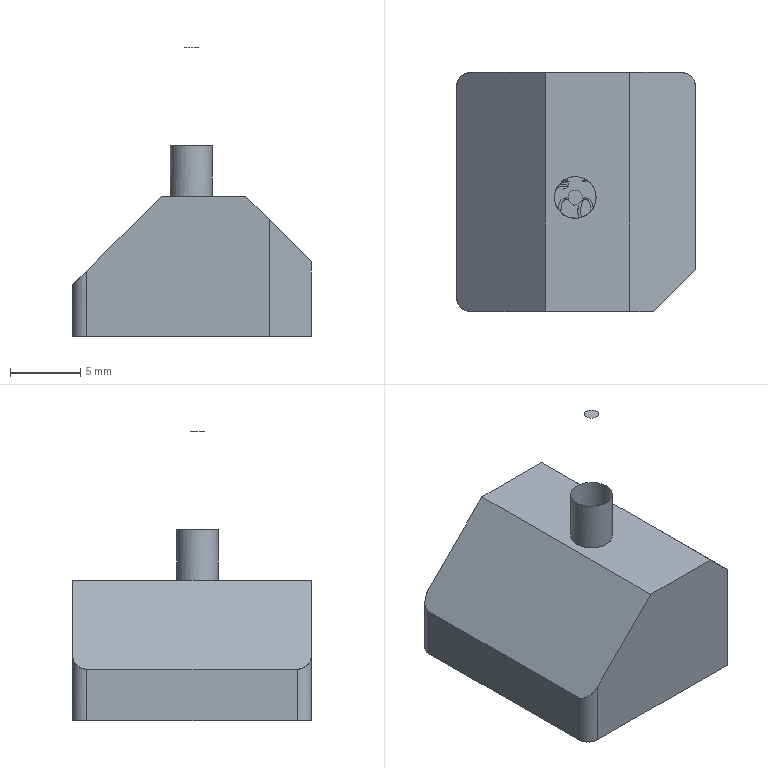NC program | PowerMill | posted with a generic post | part box 17 x 17 x 20.603 mm
Lines 3962 to 5007 of 42778:
N4059 M6
N4060 S18000 M03
N4061 G00 G90 X0.002 Y0.0
N4062 G43 Z10.803 H14
N4063
N4064 G05 P10000 R8
N4065 X1.2168 Y-3.1988
N4066 Z0.8074
N4067 G01 Z-0.3926 F1200.0
N4068 X1.1992 Y-3.1296 F2000.0
N4069 X1.174 Y-3.0627
N4070 X1.1415 Y-2.9991
N4071 X1.102 Y-2.9395
N4072 X1.0562 Y-2.8847
N4073 X1.0046 Y-2.8353
N4074 X0.9478 Y-2.792
N4075 X0.8865 Y-2.7553
N4076 X0.8215 Y-2.7256
N4077 X0.7536 Y-2.7034
N4078 X0.6836 Y-2.6889
N4079 X0.6124 Y-2.6823
N4080 X0.541 Y-2.6836
N4081 X0.4702 Y-2.6929
N4082 X0.4657 Y-2.6938
N4083 X0.3401 Y-2.7184
N4084 X0.2083 Y-2.7366
N4085 X0.0731 Y-2.7478
N4086 X-0.0548 Y-2.7513
N4087 X-0.1828 Y-2.7476
N4088 X-0.3196 Y-2.7359
N4089 X-0.4555 Y-2.7162
N4090 X-0.5901 Y-2.6887
N4091 X-0.7228 Y-2.6534
N4092 X-0.8532 Y-2.6105
N4093 X-0.9809 Y-2.56
N4094 X-1.1048 Y-2.5025
N4095 X-1.2252 Y-2.4378
N4096 X-1.3415 Y-2.3664
N4097 X-1.4534 Y-2.2882
N4098 X-1.5606 Y-2.2037
N4099 X-1.6629 Y-2.113
N4100 X-1.7598 Y-2.0163
N4101 X-1.8511 Y-1.914
N4102 X-1.9364 Y-1.8064
N4103 X-2.0154 Y-1.694
N4104 X-2.0876 Y-1.5772
N4105 X-2.1529 Y-1.4566
N4106 X-2.211 Y-1.3325
N4107 X-2.2616 Y-1.2056
N4108 X-2.3048 Y-1.0759
N4109 X-2.3403 Y-0.944
N4110 X-2.3672 Y-0.8149
N4111 X-2.3868 Y-0.6833
N4112 X-2.3991 Y-0.5473
N4113 X-2.4036 Y-0.4091
N4114 X-2.4002 Y-0.2725
N4115 X-2.3892 Y-0.1398
N4116 X-2.371 Y-0.0105
N4117 X-2.3454 Y0.1205
N4118 X-2.3121 Y0.2505
N4119 X-2.2717 Y0.3769
N4120 X-2.2247 Y0.4992
N4121 X-2.171 Y0.6193
N4122 X-2.1083 Y0.7407
N4123 X-2.0386 Y0.8582
N4124 X-1.9622 Y0.9715
N4125 X-1.8793 Y1.0801
N4126 X-1.7902 Y1.1838
N4127 X-1.6951 Y1.2823
N4128 X-1.5943 Y1.3751
N4129 X-1.4883 Y1.4619
N4130 X-1.3773 Y1.5424
N4131 X-1.262 Y1.6162
N4132 X-1.1426 Y1.6832
N4133 X-1.0197 Y1.743
N4134 X-0.8935 Y1.7956
N4135 X-0.7645 Y1.8407
N4136 X-0.6331 Y1.8783
N4137 X-0.4997 Y1.9082
N4138 X-0.3645 Y1.9303
N4139 X-0.2281 Y1.9446
N4140 X-0.0912 Y1.9509
N4141 X0.0459 Y1.9492
N4142 X0.1824 Y1.9395
N4143 X0.3181 Y1.9219
N4144 X0.4525 Y1.8964
N4145 X0.585 Y1.8632
N4146 X0.7152 Y1.8224
N4147 X0.8428 Y1.7741
N4148 X0.9676 Y1.7184
N4149 X1.089 Y1.6556
N4150 X1.2066 Y1.5857
N4151 X1.3201 Y1.509
N4152 X1.429 Y1.4258
N4153 X1.5329 Y1.3364
N4154 X1.6315 Y1.241
N4155 X1.7242 Y1.1402
N4156 X1.8108 Y1.0342
N4157 X1.891 Y0.9235
N4158 X1.9646 Y0.8085
N4159 X2.0312 Y0.6894
N4160 X2.0909 Y0.5668
N4161 X2.1433 Y0.441
N4162 X2.1883 Y0.3124
N4163 X2.2259 Y0.1811
N4164 X2.2559 Y0.0475
N4165 X2.2781 Y-0.0877
N4166 X2.2924 Y-0.2239
N4167 X2.2987 Y-0.3607
N4168 X2.297 Y-0.4977
N4169 X2.2873 Y-0.6344
N4170 X2.2697 Y-0.7703
N4171 X2.2442 Y-0.9049
N4172 X2.2109 Y-1.0377
N4173 X2.1699 Y-1.1684
N4174 X2.1213 Y-1.2965
N4175 X2.0654 Y-1.4214
N4176 X2.0024 Y-1.5429
N4177 X1.9324 Y-1.6605
N4178 X1.8557 Y-1.7738
N4179 X1.7725 Y-1.8824
N4180 X1.6832 Y-1.9861
N4181 X1.5878 Y-2.0845
N4182 X1.4868 Y-2.1772
N4183 X1.3805 Y-2.264
N4184 X1.2693 Y-2.3444
N4185 X1.1538 Y-2.4182
N4186 X1.0342 Y-2.485
N4187 X0.9111 Y-2.5448
N4188 X0.7847 Y-2.5972
N4189 X0.6555 Y-2.6423
N4190 X0.5239 Y-2.6798
N4191 X0.4657 Y-2.6938
N4192 X0.3973 Y-2.7143
N4193 X0.3316 Y-2.7423
N4194 X0.2694 Y-2.7775
N4195 X0.2115 Y-2.8194
N4196 X0.1587 Y-2.8675
N4197 X0.1115 Y-2.9212
N4198 X0.0707 Y-2.9798
N4199 X0.0366 Y-3.0426
N4200 X0.0097 Y-3.1088
N4201 X-0.0096 Y-3.1775
N4202 X-0.0212 Y-3.2481
N4203 X-0.0248 Y-3.3195
N4204 X-0.0204 Y-3.3907
N4205 X-0.0081 Y-3.4611
N4206 X-0.0071 Y-3.4656
N4207 X1.2241 Y-3.1952 Z-0.4404
N4208 X1.2056 Y-3.1262
N4209 X1.1796 Y-3.0597
N4210 X1.1463 Y-2.9965
N4211 X1.1061 Y-2.9373
N4212 X1.0597 Y-2.8831
N4213 X1.0074 Y-2.8343
N4214 X0.9501 Y-2.7917
N4215 X0.8884 Y-2.7558
N4216 X0.823 Y-2.7269
N4217 X0.7549 Y-2.7055
N4218 X0.6847 Y-2.6919
N4219 X0.6135 Y-2.6861
N4220 X0.5421 Y-2.6883
N4221 X0.4714 Y-2.6985
N4222 X0.4669 Y-2.6994
N4223 X0.3618 Y-2.7213
N4224 X0.226 Y-2.7415
N4225 X0.0894 Y-2.7537
N4226 X-0.0478 Y-2.7579
N4227 X-0.185 Y-2.7542
N4228 X-0.3217 Y-2.7424
N4229 X-0.4575 Y-2.7227
N4230 X-0.5916 Y-2.6953
N4231 X-0.7235 Y-2.6602
N4232 X-0.8531 Y-2.6177
N4233 X-0.98 Y-2.5677
N4234 X-1.1039 Y-2.5104
N4235 X-1.2244 Y-2.446
N4236 X-1.341 Y-2.3746
N4237 X-1.4535 Y-2.2965
N4238 X-1.5614 Y-2.2118
N4239 X-1.6642 Y-2.121
N4240 X-1.7617 Y-2.0242
N4241 X-1.8534 Y-1.9219
N4242 X-1.939 Y-1.8145
N4243 X-2.018 Y-1.7025
N4244 X-2.0904 Y-1.5862
N4245 X-2.1557 Y-1.466
N4246 X-2.214 Y-1.3424
N4247 X-2.2649 Y-1.2158
N4248 X-2.3083 Y-1.0865
N4249 X-2.3442 Y-0.9549
N4250 X-2.3725 Y-0.8213
N4251 X-2.3931 Y-0.6857
N4252 X-2.4058 Y-0.5492
N4253 X-2.4105 Y-0.412
N4254 X-2.4072 Y-0.2748
N4255 X-2.3959 Y-0.1382
N4256 X-2.3767 Y-0.0025
N4257 X-2.3497 Y0.1316
N4258 X-2.315 Y0.2638
N4259 X-2.2727 Y0.3938
N4260 X-2.223 Y0.5212
N4261 X-2.1658 Y0.6457
N4262 X-2.1015 Y0.7667
N4263 X-2.0302 Y0.8838
N4264 X-1.9522 Y0.9967
N4265 X-1.8677 Y1.105
N4266 X-1.777 Y1.2081
N4267 X-1.6807 Y1.3056
N4268 X-1.5789 Y1.3973
N4269 X-1.472 Y1.4828
N4270 X-1.3606 Y1.5618
N4271 X-1.2448 Y1.6342
N4272 X-1.1251 Y1.6997
N4273 X-1.0019 Y1.7581
N4274 X-0.8755 Y1.8093
N4275 X-0.7463 Y1.8532
N4276 X-0.6144 Y1.8897
N4277 X-0.4804 Y1.9187
N4278 X-0.3453 Y1.9397
N4279 X-0.2094 Y1.9529
N4280 X-0.0731 Y1.958
N4281 X0.0635 Y1.9552
N4282 X0.2001 Y1.9444
N4283 X0.3363 Y1.9256
N4284 X0.4719 Y1.8988
N4285 X0.6034 Y1.865
N4286 X0.7329 Y1.8235
N4287 X0.8602 Y1.7744
N4288 X0.9847 Y1.7178
N4289 X1.106 Y1.6538
N4290 X1.2238 Y1.5827
N4291 X1.3375 Y1.5048
N4292 X1.4453 Y1.4212
N4293 X1.5484 Y1.3313
N4294 X1.6461 Y1.2356
N4295 X1.7381 Y1.1342
N4296 X1.8243 Y1.0275
N4297 X1.9042 Y0.9158
N4298 X1.9776 Y0.7995
N4299 X2.044 Y0.6792
N4300 X2.1033 Y0.5553
N4301 X2.1553 Y0.4284
N4302 X2.1997 Y0.2989
N4303 X2.2364 Y0.1672
N4304 X2.2655 Y0.0335
N4305 X2.2868 Y-0.1019
N4306 X2.3001 Y-0.2384
N4307 X2.3056 Y-0.3755
N4308 X2.303 Y-0.5128
N4309 X2.2925 Y-0.6495
N4310 X2.274 Y-0.7854
N4311 X2.2476 Y-0.9199
N4312 X2.2135 Y-1.0527
N4313 X2.1718 Y-1.1829
N4314 X2.1226 Y-1.3107
N4315 X2.0661 Y-1.4354
N4316 X2.0024 Y-1.5566
N4317 X1.9318 Y-1.674
N4318 X1.8544 Y-1.7872
N4319 X1.7705 Y-1.8957
N4320 X1.6804 Y-1.9991
N4321 X1.5845 Y-2.0972
N4322 X1.4831 Y-2.1894
N4323 X1.3765 Y-2.2756
N4324 X1.2651 Y-2.3554
N4325 X1.1492 Y-2.4286
N4326 X1.0293 Y-2.4951
N4327 X0.9058 Y-2.5545
N4328 X0.7801 Y-2.6062
N4329 X0.6511 Y-2.6506
N4330 X0.5189 Y-2.6877
N4331 X0.4961 Y-2.6933
N4332 X0.4669 Y-2.6994
N4333 X0.3979 Y-2.7179
N4334 X0.3314 Y-2.7439
N4335 X0.2682 Y-2.7772
N4336 X0.209 Y-2.8174
N4337 X0.1548 Y-2.8638
N4338 X0.106 Y-2.9161
N4339 X0.0634 Y-2.9734
N4340 X0.0275 Y-3.0351
N4341 X-0.0014 Y-3.1005
N4342 X-0.0228 Y-3.1686
N4343 X-0.0365 Y-3.2388
N4344 X-0.0422 Y-3.31
N4345 X-0.04 Y-3.3814
N4346 X-0.0298 Y-3.4521
N4347 X-0.0289 Y-3.4566
N4348 X1.2313 Y-3.1926 Z-0.4882
N4349 X1.212 Y-3.1238
N4350 X1.1852 Y-3.0576
N4351 X1.1511 Y-2.9948
N4352 X1.1103 Y-2.9361
N4353 X1.0632 Y-2.8824
N4354 X1.0104 Y-2.8343
N4355 X0.9525 Y-2.7924
N4356 X0.8904 Y-2.7571
N4357 X0.8247 Y-2.7291
N4358 X0.7563 Y-2.7085
N4359 X0.686 Y-2.6956
N4360 X0.6147 Y-2.6907
N4361 X0.5433 Y-2.6938
N4362 X0.4728 Y-2.7047
N4363 X0.4683 Y-2.7057
N4364 X0.3906 Y-2.7229
N4365 X0.255 Y-2.7447
N4366 X0.1183 Y-2.7585
N4367 X-0.019 Y-2.7644
N4368 X-0.1565 Y-2.7623
N4369 X-0.2936 Y-2.7522
N4370 X-0.4299 Y-2.7342
N4371 X-0.5648 Y-2.7084
N4372 X-0.698 Y-2.6747
N4373 X-0.829 Y-2.6334
N4374 X-0.9574 Y-2.5845
N4375 X-1.0827 Y-2.5283
N4376 X-1.2046 Y-2.4648
N4377 X-1.3227 Y-2.3944
N4378 X-1.4365 Y-2.3172
N4379 X-1.5456 Y-2.2335
N4380 X-1.6496 Y-2.1437
N4381 X-1.7481 Y-2.048
N4382 X-1.841 Y-1.9468
N4383 X-1.9278 Y-1.8403
N4384 X-2.0083 Y-1.729
N4385 X-2.0822 Y-1.6132
N4386 X-2.1492 Y-1.4934
N4387 X-2.2092 Y-1.3698
N4388 X-2.2618 Y-1.243
N4389 X-2.3071 Y-1.1133
N4390 X-2.3447 Y-0.9812
N4391 X-2.3746 Y-0.847
N4392 X-2.3966 Y-0.7113
N4393 X-2.4108 Y-0.5747
N4394 X-2.4169 Y-0.4375
N4395 X-2.4151 Y-0.3001
N4396 X-2.4053 Y-0.1632
N4397 X-2.3876 Y-0.027
N4398 X-2.362 Y0.1076
N4399 X-2.3288 Y0.2404
N4400 X-2.2879 Y0.371
N4401 X-2.2396 Y0.499
N4402 X-2.184 Y0.624
N4403 X-2.1211 Y0.7457
N4404 X-2.0512 Y0.8637
N4405 X-1.9745 Y0.9775
N4406 X-1.8912 Y1.0868
N4407 X-1.8016 Y1.1912
N4408 X-1.7061 Y1.2902
N4409 X-1.6051 Y1.3835
N4410 X-1.499 Y1.4706
N4411 X-1.3881 Y1.5513
N4412 X-1.2729 Y1.6254
N4413 X-1.1537 Y1.6926
N4414 X-1.0308 Y1.7527
N4415 X-0.9046 Y1.8056
N4416 X-0.7755 Y1.8512
N4417 X-0.6442 Y1.8892
N4418 X-0.5097 Y1.9198
N4419 X-0.3741 Y1.9426
N4420 X-0.2376 Y1.9574
N4421 X-0.1006 Y1.9643
N4422 X0.0364 Y1.9631
N4423 X0.1731 Y1.954
N4424 X0.3092 Y1.9369
N4425 X0.4441 Y1.9119
N4426 X0.577 Y1.8794
N4427 X0.7078 Y1.8391
N4428 X0.8361 Y1.7914
N4429 X0.9614 Y1.7363
N4430 X1.0834 Y1.6741
N4431 X1.2016 Y1.6048
N4432 X1.3158 Y1.5286
N4433 X1.4255 Y1.4459
N4434 X1.5303 Y1.3569
N4435 X1.6298 Y1.2619
N4436 X1.7235 Y1.1613
N4437 X1.8112 Y1.0556
N4438 X1.8925 Y0.945
N4439 X1.9672 Y0.83
N4440 X2.035 Y0.7111
N4441 X2.0958 Y0.5885
N4442 X2.1493 Y0.4626
N4443 X2.1956 Y0.3338
N4444 X2.2343 Y0.2024
N4445 X2.2654 Y0.0688
N4446 X2.2887 Y-0.0664
N4447 X2.3041 Y-0.2027
N4448 X2.3116 Y-0.3396
N4449 X2.3111 Y-0.477
N4450 X2.3026 Y-0.6142
N4451 X2.2862 Y-0.7508
N4452 X2.2618 Y-0.8862
N4453 X2.2297 Y-1.0199
N4454 X2.1899 Y-1.1512
N4455 X2.1426 Y-1.28
N4456 X2.0878 Y-1.4059
N4457 X2.0259 Y-1.5283
N4458 X1.9568 Y-1.6471
N4459 X1.8809 Y-1.7617
N4460 X1.7985 Y-1.8717
N4461 X1.7098 Y-1.9767
N4462 X1.6152 Y-2.0765
N4463 X1.5148 Y-2.1706
N4464 X1.4092 Y-2.2587
N4465 X1.2987 Y-2.3405
N4466 X1.1837 Y-2.4157
N4467 X1.0645 Y-2.4842
N4468 X0.9416 Y-2.5456
N4469 X0.8159 Y-2.5996
N4470 X0.6871 Y-2.6462
N4471 X0.5555 Y-2.6853
N4472 X0.5248 Y-2.6932
N4473 X0.4683 Y-2.7057
N4474 X0.3995 Y-2.725
N4475 X0.3333 Y-2.7518
N4476 X0.2705 Y-2.7859
N4477 X0.2118 Y-2.8267
N4478 X0.1581 Y-2.8738
N4479 X0.11 Y-2.9266
N4480 X0.0681 Y-2.9845
N4481 X0.0328 Y-3.0466
N4482 X0.0048 Y-3.1123
N4483 X-0.0158 Y-3.1807
N4484 X-0.0287 Y-3.251
N4485 X-0.0336 Y-3.3223
N4486 X-0.0305 Y-3.3937
N4487 X-0.0195 Y-3.4642
N4488 X-0.0186 Y-3.4687
N4489 X1.2384 Y-3.1902 Z-0.536
N4490 X1.2183 Y-3.1217
N4491 X1.1907 Y-3.0558
N4492 X1.156 Y-2.9934
N4493 X1.1144 Y-2.9352
N4494 X1.0667 Y-2.882
N4495 X1.0134 Y-2.8345
N4496 X0.955 Y-2.7933
N4497 X0.8925 Y-2.7587
N4498 X0.8265 Y-2.7314
N4499 X0.7578 Y-2.7116
N4500 X0.6874 Y-2.6996
N4501 X0.616 Y-2.6955
N4502 X0.5447 Y-2.6994
N4503 X0.4743 Y-2.7112
N4504 X0.4698 Y-2.7122
N4505 X0.4181 Y-2.7243
N4506 X0.2828 Y-2.7476
N4507 X0.1464 Y-2.7631
N4508 X0.0091 Y-2.7706
N4509 X-0.1286 Y-2.7701
N4510 X-0.2662 Y-2.7617
N4511 X-0.403 Y-2.7452
N4512 X-0.5387 Y-2.7209
N4513 X-0.6715 Y-2.6891
N4514 X-0.8025 Y-2.6495
N4515 X-0.9315 Y-2.6023
N4516 X-1.0579 Y-2.5474
N4517 X-1.1811 Y-2.4852
N4518 X-1.3007 Y-2.4159
N4519 X-1.4159 Y-2.3399
N4520 X-1.5264 Y-2.2575
N4521 X-1.6317 Y-2.1691
N4522 X-1.7314 Y-2.075
N4523 X-1.8251 Y-1.9756
N4524 X-1.9127 Y-1.8711
N4525 X-1.9944 Y-1.7614
N4526 X-2.0699 Y-1.6464
N4527 X-2.1389 Y-1.5269
N4528 X-2.2011 Y-1.4033
N4529 X-2.2559 Y-1.2765
N4530 X-2.3031 Y-1.1472
N4531 X-2.3426 Y-1.016
N4532 X-2.3742 Y-0.8833
N4533 X-2.3983 Y-0.7477
N4534 X-2.4145 Y-0.6109
N4535 X-2.4228 Y-0.4735
N4536 X-2.423 Y-0.3357
N4537 X-2.4153 Y-0.1983
N4538 X-2.3996 Y-0.0614
N4539 X-2.376 Y0.0742
N4540 X-2.3447 Y0.2078
N4541 X-2.3057 Y0.3393
N4542 X-2.2593 Y0.4682
N4543 X-2.2054 Y0.5943
N4544 X-2.1443 Y0.7171
N4545 X-2.0762 Y0.8362
N4546 X-2.0011 Y0.9514
N4547 X-1.9194 Y1.0621
N4548 X-1.8314 Y1.168
N4549 X-1.7373 Y1.2687
N4550 X-1.6376 Y1.3636
N4551 X-1.5327 Y1.4526
N4552 X-1.4229 Y1.5352
N4553 X-1.3087 Y1.6113
N4554 X-1.1903 Y1.6805
N4555 X-1.0682 Y1.7427
N4556 X-0.9427 Y1.7978
N4557 X-0.8141 Y1.8455
N4558 X-0.6829 Y1.8858
N4559 X-0.5493 Y1.9185
N4560 X-0.4139 Y1.9435
N4561 X-0.2773 Y1.9606
N4562 X-0.1398 Y1.9697
N4563 X-0.0022 Y1.9708
N4564 X0.1352 Y1.964
N4565 X0.2718 Y1.9492
N4566 X0.4074 Y1.9265
N4567 X0.5414 Y1.8959
N4568 X0.6734 Y1.8576
N4569 X0.8031 Y1.8118
N4570 X0.9299 Y1.7584
N4571 X1.0533 Y1.6978
N4572 X1.1731 Y1.6302
N4573 X1.2888 Y1.5556
N4574 X1.4001 Y1.4745
N4575 X1.5065 Y1.387
N4576 X1.6075 Y1.2935
N4577 X1.7029 Y1.1944
N4578 X1.7925 Y1.09
N4579 X1.8757 Y0.9805
N4580 X1.9525 Y0.8664
N4581 X2.0226 Y0.748
N4582 X2.0857 Y0.6258
N4583 X2.1416 Y0.5001
N4584 X2.19 Y0.3714
N4585 X2.231 Y0.2402
N4586 X2.2643 Y0.1067
N4587 X2.2898 Y-0.0285
N4588 X2.3074 Y-0.165
N4589 X2.317 Y-0.3024
N4590 X2.3187 Y-0.44
N4591 X2.3124 Y-0.5774
N4592 X2.2982 Y-0.7142
N4593 X2.276 Y-0.8499
N4594 X2.246 Y-0.9841
N4595 X2.2083 Y-1.1164
N4596 X2.1629 Y-1.2462
N4597 X2.1101 Y-1.3733
N4598 X2.05 Y-1.497
N4599 X1.9829 Y-1.6171
N4600 X1.9088 Y-1.7331
N4601 X1.8282 Y-1.8446
N4602 X1.7411 Y-1.9513
N4603 X1.6481 Y-2.0527
N4604 X1.5494 Y-2.1485
N4605 X1.4453 Y-2.2385
N4606 X1.3361 Y-2.3222
N4607 X1.2226 Y-2.3993
N4608 X1.1042 Y-2.4702
N4609 X0.9828 Y-2.5336
N4610 X0.8581 Y-2.5898
N4611 X0.7302 Y-2.6386
N4612 X0.599 Y-2.6802
N4613 X0.5518 Y-2.6931
N4614 X0.4698 Y-2.7122
N4615 X0.4013 Y-2.7323
N4616 X0.3354 Y-2.7599
N4617 X0.273 Y-2.7947
N4618 X0.2148 Y-2.8362
N4619 X0.1616 Y-2.8839
N4620 X0.1141 Y-2.9373
N4621 X0.0729 Y-2.9956
N4622 X0.0383 Y-3.0582
N4623 X0.011 Y-3.1242
N4624 X-0.0088 Y-3.1928
N4625 X-0.0208 Y-3.2633
N4626 X-0.0249 Y-3.3346
N4627 X-0.021 Y-3.4059
N4628 X-0.0092 Y-3.4764
N4629 X-0.0082 Y-3.4808
N4630 X1.2448 Y-3.1895 Z-0.5838
N4631 X1.224 Y-3.1211
N4632 X1.1958 Y-3.0555
N4633 X1.1604 Y-2.9934
N4634 X1.1183 Y-2.9356
N4635 X1.07 Y-2.883
N4636 X1.0162 Y-2.836
N4637 X0.9575 Y-2.7953
N4638 X0.8946 Y-2.7614
N4639 X0.8283 Y-2.7348
N4640 X0.7595 Y-2.7156
N4641 X0.6889 Y-2.7043
N4642 X0.6175 Y-2.7009
N4643 X0.5463 Y-2.7055
N4644 X0.4759 Y-2.718
N4645 X0.4715 Y-2.7191
N4646 X0.4435 Y-2.7259
N4647 X0.308 Y-2.7507
N4648 X0.1712 Y-2.7676
N4649 X0.0336 Y-2.7765
N4650 X-0.1043 Y-2.7775
N4651 X-0.242 Y-2.7705
N4652 X-0.379 Y-2.7555
N4653 X-0.5149 Y-2.7326
N4654 X-0.6492 Y-2.7019
N4655 X-0.7815 Y-2.6635
N4656 X-0.9113 Y-2.6175
N4657 X-1.0382 Y-2.5641
N4658 X-1.1618 Y-2.5034
N4659 X-1.2818 Y-2.4356
N4660 X-1.3977 Y-2.3609
N4661 X-1.5091 Y-2.2797
N4662 X-1.6156 Y-2.1921
N4663 X-1.7167 Y-2.0986
N4664 X-1.8123 Y-1.9994
N4665 X-1.9019 Y-1.8949
N4666 X-1.9854 Y-1.7853
N4667 X-2.0623 Y-1.6713
N4668 X-2.1325 Y-1.553
N4669 X-2.1957 Y-1.4307
N4670 X-2.2517 Y-1.3049
N4671 X-2.3005 Y-1.1759
N4672 X-2.3417 Y-1.0442
N4673 X-2.3751 Y-0.9107
N4674 X-2.4008 Y-0.7752
N4675 X-2.4186 Y-0.6385
N4676 X-2.4285 Y-0.5011
N4677 X-2.4304 Y-0.3632
N4678 X-2.4242 Y-0.2255
N4679 X-2.4101 Y-0.0884
N4680 X-2.3881 Y0.0477
N4681 X-2.3583 Y0.182
N4682 X-2.3208 Y0.3144
N4683 X-2.2757 Y0.4442
N4684 X-2.2232 Y0.5713
N4685 X-2.1634 Y0.6951
N4686 X-2.0965 Y0.8153
N4687 X-2.0228 Y0.9316
N4688 X-1.9423 Y1.0435
N4689 X-1.8554 Y1.1507
N4690 X-1.7625 Y1.2526
N4691 X-1.6639 Y1.3489
N4692 X-1.56 Y1.4392
N4693 X-1.4511 Y1.5233
N4694 X-1.3375 Y1.601
N4695 X-1.2197 Y1.6719
N4696 X-1.0979 Y1.7359
N4697 X-0.9726 Y1.7927
N4698 X-0.8441 Y1.8423
N4699 X-0.7129 Y1.8843
N4700 X-0.5795 Y1.9188
N4701 X-0.4442 Y1.9454
N4702 X-0.3075 Y1.9642
N4703 X-0.17 Y1.9751
N4704 X-0.0323 Y1.978
N4705 X0.1053 Y1.9729
N4706 X0.2424 Y1.9598
N4707 X0.3785 Y1.9388
N4708 X0.5131 Y1.9099
N4709 X0.6458 Y1.8733
N4710 X0.776 Y1.8292
N4711 X0.9035 Y1.7776
N4712 X1.0277 Y1.7187
N4713 X1.1484 Y1.6527
N4714 X1.2651 Y1.5798
N4715 X1.3775 Y1.5002
N4716 X1.4852 Y1.4141
N4717 X1.5878 Y1.3219
N4718 X1.6849 Y1.2239
N4719 X1.7761 Y1.1205
N4720 X1.861 Y1.0122
N4721 X1.9395 Y0.8992
N4722 X2.0113 Y0.7819
N4723 X2.0762 Y0.6606
N4724 X2.1339 Y0.5358
N4725 X2.1844 Y0.4079
N4726 X2.2273 Y0.2773
N4727 X2.2626 Y0.1445
N4728 X2.2902 Y0.0097
N4729 X2.31 Y-0.1266
N4730 X2.3218 Y-0.264
N4731 X2.3257 Y-0.402
N4732 X2.3216 Y-0.54
N4733 X2.3096 Y-0.6773
N4734 X2.2896 Y-0.8136
N4735 X2.2618 Y-0.9482
N4736 X2.2263 Y-1.081
N4737 X2.1831 Y-1.2115
N4738 X2.1324 Y-1.3395
N4739 X2.0743 Y-1.4644
N4740 X2.0091 Y-1.5857
N4741 X1.9369 Y-1.7031
N4742 X1.8579 Y-1.8162
N4743 X1.7725 Y-1.9247
N4744 X1.6811 Y-2.0279
N4745 X1.5839 Y-2.1255
N4746 X1.4813 Y-2.2174
N4747 X1.3736 Y-2.3031
N4748 X1.261 Y-2.3825
N4749 X1.1441 Y-2.4552
N4750 X1.023 Y-2.5211
N4751 X0.8984 Y-2.5799
N4752 X0.7706 Y-2.6313
N4753 X0.64 Y-2.6752
N4754 X0.5775 Y-2.6933
N4755 X0.4715 Y-2.7191
N4756 X0.4031 Y-2.7398
N4757 X0.3375 Y-2.7681
N4758 X0.2755 Y-2.8035
N4759 X0.2177 Y-2.8456
N4760 X0.165 Y-2.8938
N4761 X0.118 Y-2.9477
N4762 X0.0773 Y-3.0064
N4763 X0.0435 Y-3.0693
N4764 X0.0168 Y-3.1355
N4765 X-0.0023 Y-3.2044
N4766 X-0.0136 Y-3.275
N4767 X-0.017 Y-3.3463
N4768 X-0.0124 Y-3.4176
N4769 X0.0001 Y-3.4879
N4770 X0.0011 Y-3.4924
N4771 X1.2513 Y-3.1886 Z-0.6317
N4772 X1.2298 Y-3.1205
N4773 X1.2009 Y-3.0552
N4774 X1.1649 Y-2.9935
N4775 X1.1222 Y-2.9361
N4776 X1.0734 Y-2.8839
N4777 X1.0191 Y-2.8375
N4778 X0.96 Y-2.7974
N4779 X0.8968 Y-2.7642
N4780 X0.8303 Y-2.7382
N4781 X0.7612 Y-2.7198
N4782 X0.6905 Y-2.7091
N4783 X0.6191 Y-2.7065
N4784 X0.5479 Y-2.7118
N4785 X0.4777 Y-2.725
N4786 X0.4733 Y-2.7261
N4787 X0.4683 Y-2.7274
N4788 X0.3329 Y-2.7536
N4789 X0.1962 Y-2.7719
N4790 X0.0587 Y-2.7822
N4791 X-0.0794 Y-2.7846
N4792 X-0.2173 Y-2.779
N4793 X-0.3548 Y-2.7654
N4794 X-0.4911 Y-2.7439
N4795 X-0.6259 Y-2.7146
N4796 X-0.7585 Y-2.6777
N4797 X-0.8887 Y-2.6332
N4798 X-1.016 Y-2.5814
N4799 X-1.1402 Y-2.5222
N4800 X-1.2607 Y-2.456
N4801 X-1.3773 Y-2.3829
N4802 X-1.4896 Y-2.3031
N4803 X-1.5972 Y-2.2168
N4804 X-1.6997 Y-2.1244
N4805 X-1.7968 Y-2.0261
N4806 X-1.888 Y-1.9224
N4807 X-1.9731 Y-1.8137
N4808 X-2.0516 Y-1.7004
N4809 X-2.1233 Y-1.5828
N4810 X-2.1881 Y-1.4614
N4811 X-2.2457 Y-1.3366
N4812 X-2.2961 Y-1.2087
N4813 X-2.339 Y-1.078
N4814 X-2.3741 Y-0.9459
N4815 X-2.4016 Y-0.8118
N4816 X-2.4213 Y-0.6756
N4817 X-2.4332 Y-0.5379
N4818 X-2.4372 Y-0.3995
N4819 X-2.4331 Y-0.261
N4820 X-2.4211 Y-0.1233
N4821 X-2.4013 Y0.013
N4822 X-2.3737 Y0.1472
N4823 X-2.3385 Y0.2793
N4824 X-2.2956 Y0.4099
N4825 X-2.2452 Y0.5378
N4826 X-2.1875 Y0.6627
N4827 X-2.1226 Y0.784
N4828 X-2.0508 Y0.9015
N4829 X-1.9722 Y1.0149
N4830 X-1.8871 Y1.1235
N4831 X-1.7958 Y1.2272
N4832 X-1.6987 Y1.3254
N4833 X-1.5961 Y1.4177
N4834 X-1.4885 Y1.5039
N4835 X-1.3762 Y1.5837
N4836 X-1.2596 Y1.6567
N4837 X-1.139 Y1.7228
N4838 X-1.0149 Y1.7819
N4839 X-0.8875 Y1.8337
N4840 X-0.7573 Y1.8781
N4841 X-0.6247 Y1.9149
N4842 X-0.4898 Y1.9442
N4843 X-0.3534 Y1.9656
N4844 X-0.216 Y1.9791
N4845 X-0.078 Y1.9846
N4846 X0.06 Y1.9821
N4847 X0.1975 Y1.9717
N4848 X0.3342 Y1.9533
N4849 X0.4696 Y1.9271
N4850 X0.6032 Y1.893
N4851 X0.7345 Y1.8513
N4852 X0.8631 Y1.8022
N4853 X0.9887 Y1.7456
N4854 X1.1108 Y1.6819
N4855 X1.2291 Y1.6113
N4856 X1.3432 Y1.5339
N4857 X1.4527 Y1.4499
N4858 X1.5572 Y1.3596
N4859 X1.6565 Y1.2635
N4860 X1.7499 Y1.1618
N4861 X1.8372 Y1.055
N4862 X1.9181 Y0.9434
N4863 X1.9924 Y0.8274
N4864 X2.0598 Y0.7073
N4865 X2.1203 Y0.5836
N4866 X2.1734 Y0.4565
N4867 X2.2191 Y0.327
N4868 X2.2571 Y0.1951
N4869 X2.2875 Y0.061
N4870 X2.3102 Y-0.075
N4871 X2.325 Y-0.2123
N4872 X2.3318 Y-0.3505
N4873 X2.3307 Y-0.4889
N4874 X2.3216 Y-0.627
N4875 X2.3046 Y-0.764
N4876 X2.2797 Y-0.8995
N4877 X2.2471 Y-1.033
N4878 X2.2069 Y-1.1643
N4879 X2.1592 Y-1.293
N4880 X2.1038 Y-1.4192
N4881 X2.0413 Y-1.542
N4882 X1.9717 Y-1.6612
N4883 X1.8952 Y-1.7763
N4884 X1.8121 Y-1.8868
N4885 X1.7228 Y-1.9923
N4886 X1.6277 Y-2.0924
N4887 X1.527 Y-2.1867
N4888 X1.4211 Y-2.2751
N4889 X1.3104 Y-2.3571
N4890 X1.1952 Y-2.4326
N4891 X1.0757 Y-2.5012
N4892 X0.9524 Y-2.5629
N4893 X0.8256 Y-2.6174
N4894 X0.6959 Y-2.6645
N4895 X0.602 Y-2.6934
N4896 X0.4733 Y-2.7261
N4897 X0.4051 Y-2.7475
N4898 X0.3398 Y-2.7764
N4899 X0.2781 Y-2.8124
N4900 X0.2207 Y-2.8551
N4901 X0.1685 Y-2.9039
N4902 X0.1221 Y-2.9582
N4903 X0.082 Y-3.0173
N4904 X0.0488 Y-3.0806
N4905 X0.0228 Y-3.1471
N4906 X0.0044 Y-3.2161
N4907 X-0.0062 Y-3.2868
N4908 X-0.0089 Y-3.3582
N4909 X-0.0036 Y-3.4295
N4910 X0.0096 Y-3.4997
N4911 X0.0107 Y-3.5041
N4912 X1.2312 Y-3.2288 Z-0.6795
N4913 X1.2128 Y-3.1598
N4914 X1.1869 Y-3.0932
N4915 X1.1536 Y-3.03
N4916 X1.1135 Y-2.9708
N4917 X1.0671 Y-2.9165
N4918 X1.0149 Y-2.8677
N4919 X0.9576 Y-2.825
N4920 X0.896 Y-2.789
N4921 X0.8306 Y-2.7601
N4922 X0.7625 Y-2.7386
N4923 X0.6923 Y-2.7249
N4924 X0.6211 Y-2.7191
N4925 X0.5497 Y-2.7212
N4926 X0.479 Y-2.7313
N4927 X0.4745 Y-2.7322
N4928 X0.3732 Y-2.7532
N4929 X0.2389 Y-2.7737
N4930 X0.1122 Y-2.7861
N4931 X-0.015 Y-2.7913
N4932 X-0.153 Y-2.7894
N4933 X-0.2906 Y-2.7795
N4934 X-0.4274 Y-2.7618
N4935 X-0.5632 Y-2.7361
N4936 X-0.6973 Y-2.7027
N4937 X-0.8294 Y-2.6615
N4938 X-0.9589 Y-2.6128
N4939 X-1.0855 Y-2.5566
N4940 X-1.2085 Y-2.4934
N4941 X-1.3275 Y-2.4231
N4942 X-1.4421 Y-2.3463
N4943 X-1.552 Y-2.263
N4944 X-1.657 Y-2.1735
N4945 X-1.7566 Y-2.0781
N4946 X-1.8506 Y-1.9771
N4947 X-1.9375 Y-1.8721
N4948 X-2.0188 Y-1.7615
N4949 X-2.094 Y-1.6457
N4950 X-2.1628 Y-1.5251
N4951 X-2.2245 Y-1.4008
N4952 X-2.2788 Y-1.2736
N4953 X-2.3253 Y-1.1443
N4954 X-2.364 Y-1.0133
N4955 X-2.3956 Y-0.8787
N4956 X-2.4193 Y-0.7426
N4957 X-2.4351 Y-0.6055
N4958 X-2.443 Y-0.4677
N4959 X-2.4429 Y-0.3296
N4960 X-2.4348 Y-0.1917
N4961 X-2.4187 Y-0.0545
N4962 X-2.3948 Y0.0816
N4963 X-2.363 Y0.2162
N4964 X-2.3235 Y0.349
N4965 X-2.2764 Y0.4792
N4966 X-2.2219 Y0.6063
N4967 X-2.1602 Y0.73
N4968 X-2.0917 Y0.8496
N4969 X-2.0164 Y0.9649
N4970 X-1.9345 Y1.0757
N4971 X-1.8461 Y1.182
N4972 X-1.7517 Y1.2829
N4973 X-1.6516 Y1.3782
N4974 X-1.5462 Y1.4676
N4975 X-1.4358 Y1.5507
N4976 X-1.3208 Y1.6274
N4977 X-1.2014 Y1.6973
N4978 X-1.0784 Y1.7602
N4979 X-0.9519 Y1.8158
N4980 X-0.8224 Y1.864
N4981 X-0.6903 Y1.9047
N4982 X-0.5561 Y1.9377
N4983 X-0.4202 Y1.9629
N4984 X-0.2831 Y1.9802
N4985 X-0.1451 Y1.9896
N4986 X-0.0068 Y1.991
N4987 X0.1313 Y1.9844
N4988 X0.2688 Y1.9699
N4989 X0.4052 Y1.9475
N4990 X0.54 Y1.9171
N4991 X0.6729 Y1.8791
N4992 X0.803 Y1.8335
N4993 X0.9302 Y1.7805
N4994 X1.0541 Y1.7203
N4995 X1.1743 Y1.6529
N4996 X1.2907 Y1.5787
N4997 X1.4027 Y1.4977
N4998 X1.5101 Y1.4103
N4999 X1.6122 Y1.3167
N5000 X1.7088 Y1.2175
N5001 X1.7994 Y1.113
N5002 X1.8837 Y1.0035
N5003 X1.9615 Y0.8896
N5004 X2.0324 Y0.7715
N5005 X2.0964 Y0.6495
N5006 X2.1533 Y0.524
N5007 X2.2028 Y0.3954
N5008 X2.2449 Y0.2641
N5009 X2.2794 Y0.1303
N5010 X2.3062 Y-0.0054
N5011 X2.3251 Y-0.1424
N5012 X2.3361 Y-0.2803
N5013 X2.3391 Y-0.4186
N5014 X2.3341 Y-0.5568
N5015 X2.3211 Y-0.6942
N5016 X2.3003 Y-0.8306
N5017 X2.2716 Y-0.9656
N5018 X2.2351 Y-1.0986
N5019 X2.191 Y-1.2294
N5020 X2.1394 Y-1.3575
N5021 X2.0805 Y-1.4823
N5022 X2.0144 Y-1.6035
N5023 X1.9414 Y-1.7208
N5024 X1.8617 Y-1.8337
N5025 X1.7755 Y-1.942
N5026 X1.6832 Y-2.0451
N5027 X1.5851 Y-2.1428
N5028 X1.4815 Y-2.2346
N5029 X1.3729 Y-2.3203
N5030 X1.2596 Y-2.3995
N5031 X1.143 Y-2.4715
N5032 X1.0222 Y-2.5367
N5033 X0.8971 Y-2.5951
N5034 X0.7683 Y-2.6464
N5035 X0.636 Y-2.6906
N5036 X0.6256 Y-2.6937
N5037 X0.5026 Y-2.7264
N5038 X0.4745 Y-2.7322
N5039 X0.4055 Y-2.7506
N5040 X0.339 Y-2.7766
N5041 X0.2757 Y-2.8098
N5042 X0.2165 Y-2.8499
N5043 X0.1622 Y-2.8963
N5044 X0.1134 Y-2.9485
N5045 X0.0708 Y-3.0058
N5046 X0.0348 Y-3.0675
N5047 X0.0058 Y-3.1328
N5048 X-0.0156 Y-3.201
N5049 X-0.0294 Y-3.2711
N5050 X-0.0352 Y-3.3423
N5051 X-0.0331 Y-3.4137
N5052 X-0.023 Y-3.4844
N5053 X-0.0221 Y-3.4889
N5054 X1.2354 Y-3.231 Z-0.7273
N5055 X1.2167 Y-3.1621
N5056 X1.1903 Y-3.0957
N5057 X1.1567 Y-3.0327
N5058 X1.1163 Y-2.9737
N5059 X1.0695 Y-2.9196
N5060 X1.0171 Y-2.8712
N5061 X0.9596 Y-2.8288
N5062 X0.8977 Y-2.7931
N5063 X0.8322 Y-2.7646
N5064 X0.7639 Y-2.7435
N5065 X0.6937 Y-2.7302
N5066 X0.6224 Y-2.7248
N5067 X0.5511 Y-2.7273
N5068 X0.4804 Y-2.7378
N5069 X0.4759 Y-2.7387
N5070 X0.3819 Y-2.7588
N5071 X0.2456 Y-2.7798
N5072 X0.1079 Y-2.7929
N5073 X-0.0306 Y-2.798
N5074 X-0.1693 Y-2.7952
N5075 X-0.3077 Y-2.7844
N5076 X-0.4451 Y-2.7656
N5077 X-0.5809 Y-2.7391
N5078 X-0.7148 Y-2.7048
N5079 X-0.8461 Y-2.663
N5080 X-0.9747 Y-2.6137
N5081 X-1.1006 Y-2.557
N5082 X-1.2231 Y-2.4931
N5083 X-1.3416 Y-2.4222
N5084 X-1.4559 Y-2.3446
N5085 X-1.5656 Y-2.2605
N5086 X-1.6704 Y-2.1702
N5087 X-1.7699 Y-2.0739
N5088 X-1.8637 Y-1.9719
N5089 X-1.9514 Y-1.8648
N5090 X-2.0327 Y-1.7528
N5091 X-2.1074 Y-1.6365
N5092 X-2.1752 Y-1.5162
N5093 X-2.2359 Y-1.3922
N5094 X-2.2894 Y-1.2649
N5095 X-2.3355 Y-1.1346
N5096 X-2.374 Y-1.0019
N5097 X-2.4049 Y-0.8671
N5098 X-2.4279 Y-0.7306
N5099 X-2.443 Y-0.5931
N5100 X-2.4501 Y-0.4549
N5101 X-2.4493 Y-0.3164
N5102 X-2.4405 Y-0.1782
N5103 X-2.4237 Y-0.0409
N5104 X-2.399 Y0.0953